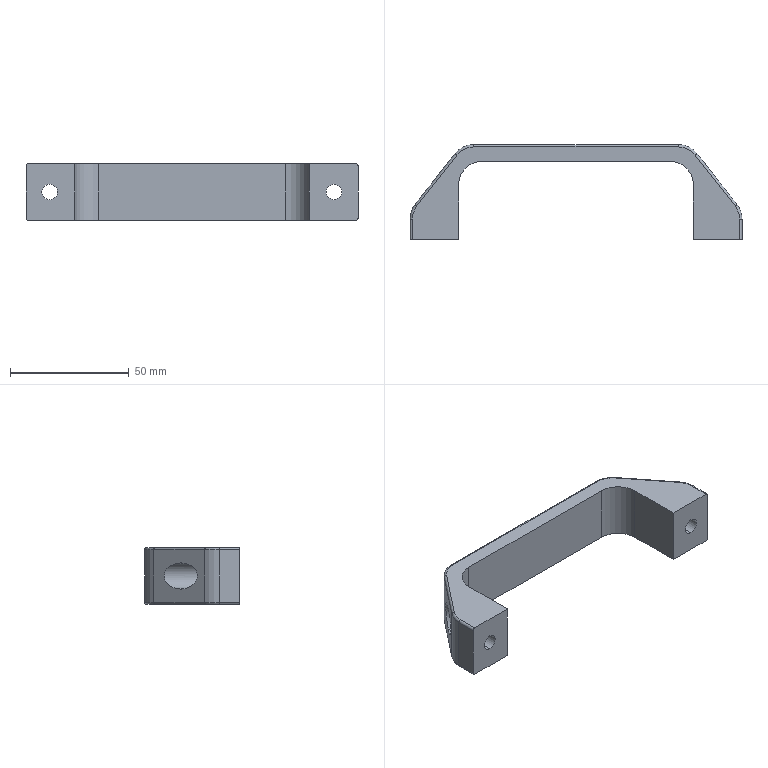Part | STEP file | Door handle | 1 solid | 46 faces | box 140 x 40 x 24 mm | volume 37832 mm3 | cylinder 24 | plane 14 | torus 8 | commonest cylinder face diameters 2 x10 20 x6 6.6 x4 11 x4